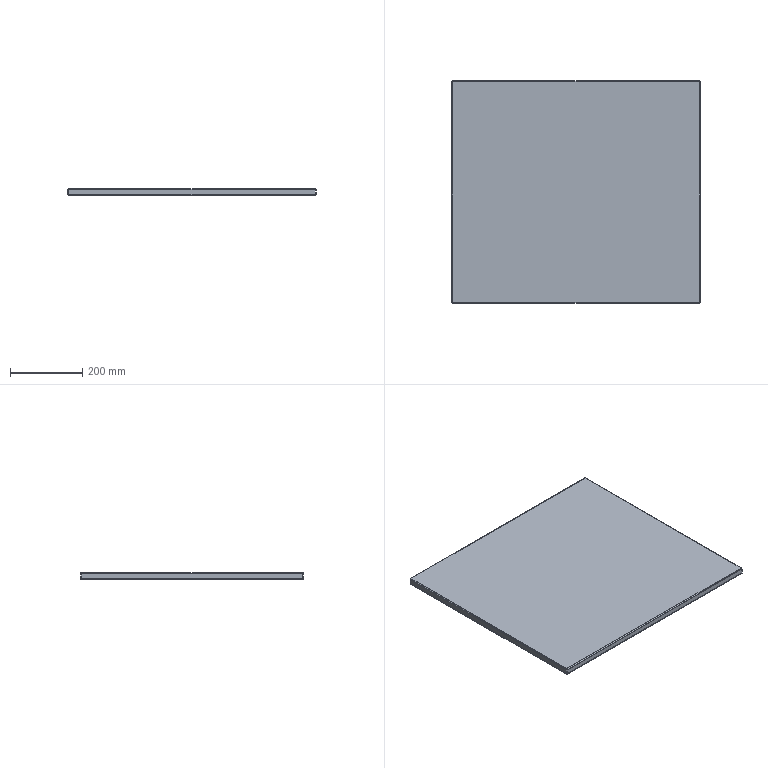Part | STEP file | Side door panel lower V1.201001 | 1 solid | 102 faces | box 686 x 615 x 19 mm | volume 731060 mm3 | cylinder 48 | plane 38 | spline 16 | commonest cylinder face diameters 3.5 x32 3 x8 6 x8